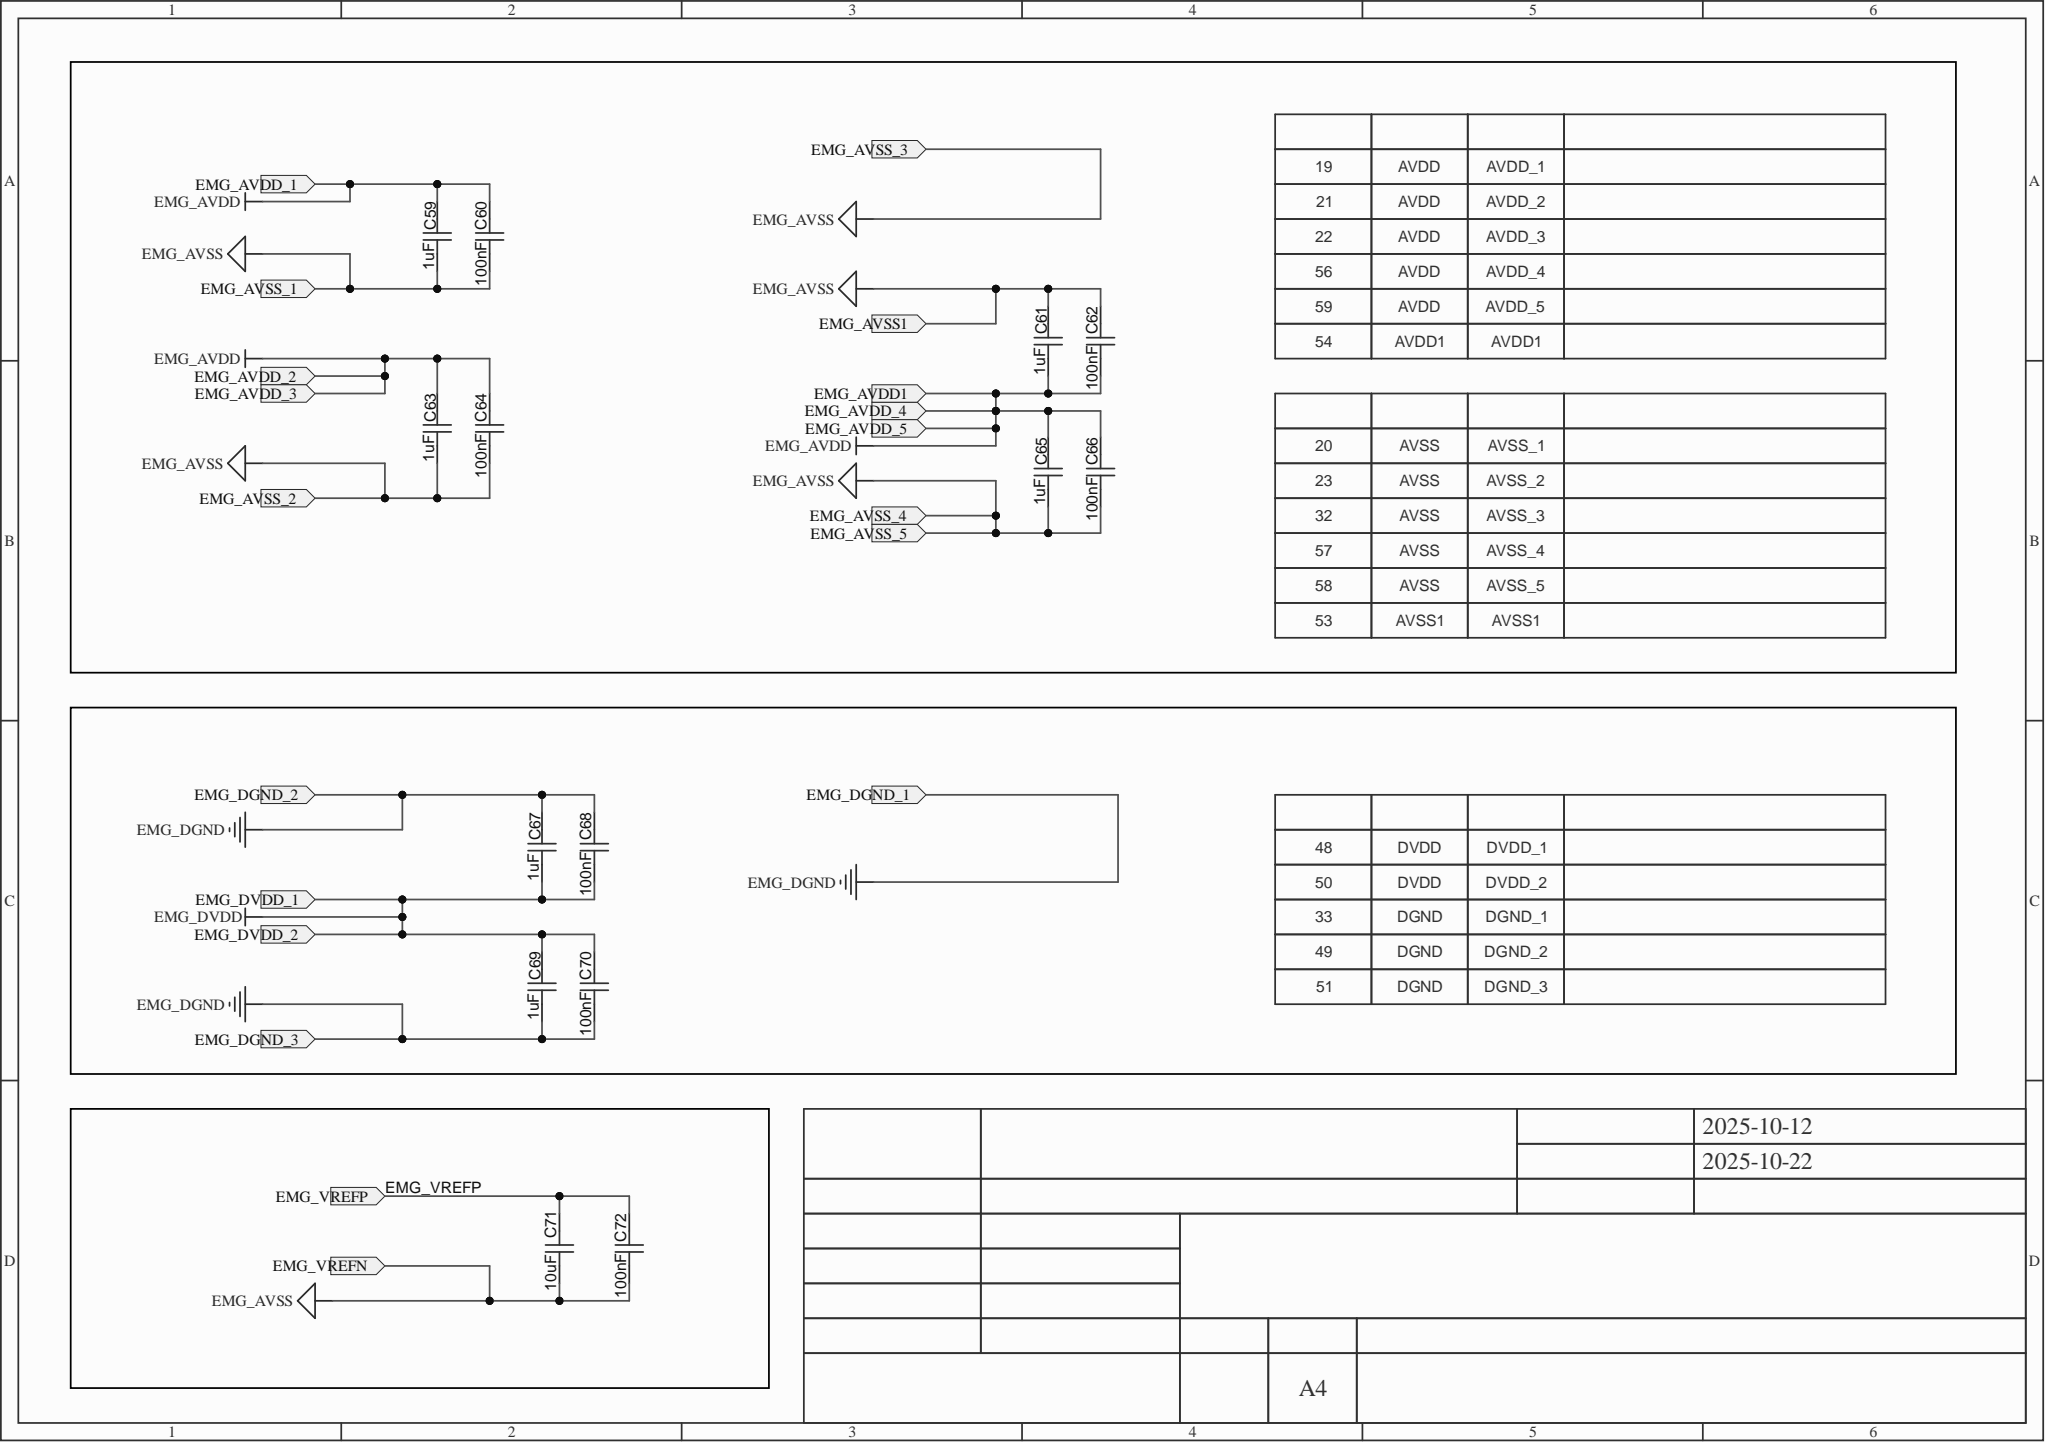Circuit board | Altium Designer | 211 parts | 126 nets | one sheet of the schematic
Parts on this sheet (reference | value | footprint):
C59 | 1uF | C0402
C60 | 100nF | C0402
C61 | 1uF | C0402
C62 | 100nF | C0402
C63 | 1uF | C0402
C64 | 100nF | C0402
C65 | 1uF | C0402
C66 | 100nF | C0402
C67 | 1uF | C0402
C68 | 100nF | C0402
C69 | 1uF | C0402
C70 | 100nF | C0402
C71 | 10uF | C0603
C72 | 100nF | C0402
Nets of these parts (net: part-pin ...):
EMG_VREFP: C71-2 C72-2
EMG_DVDD_1: C67-1 C68-1 C69-2 C70-2
EMG_DGND_1: C67-2 C68-2 C69-1 C70-1
EMG_AVSS1: C59-1 C60-1 C61-2 C62-2 C63-1 C64-1 C65-1 C66-1 C71-1 C72-1
EMG_AVDD1: C59-2 C60-2 C61-1 C62-1 C63-2 C64-2 C65-2 C66-2